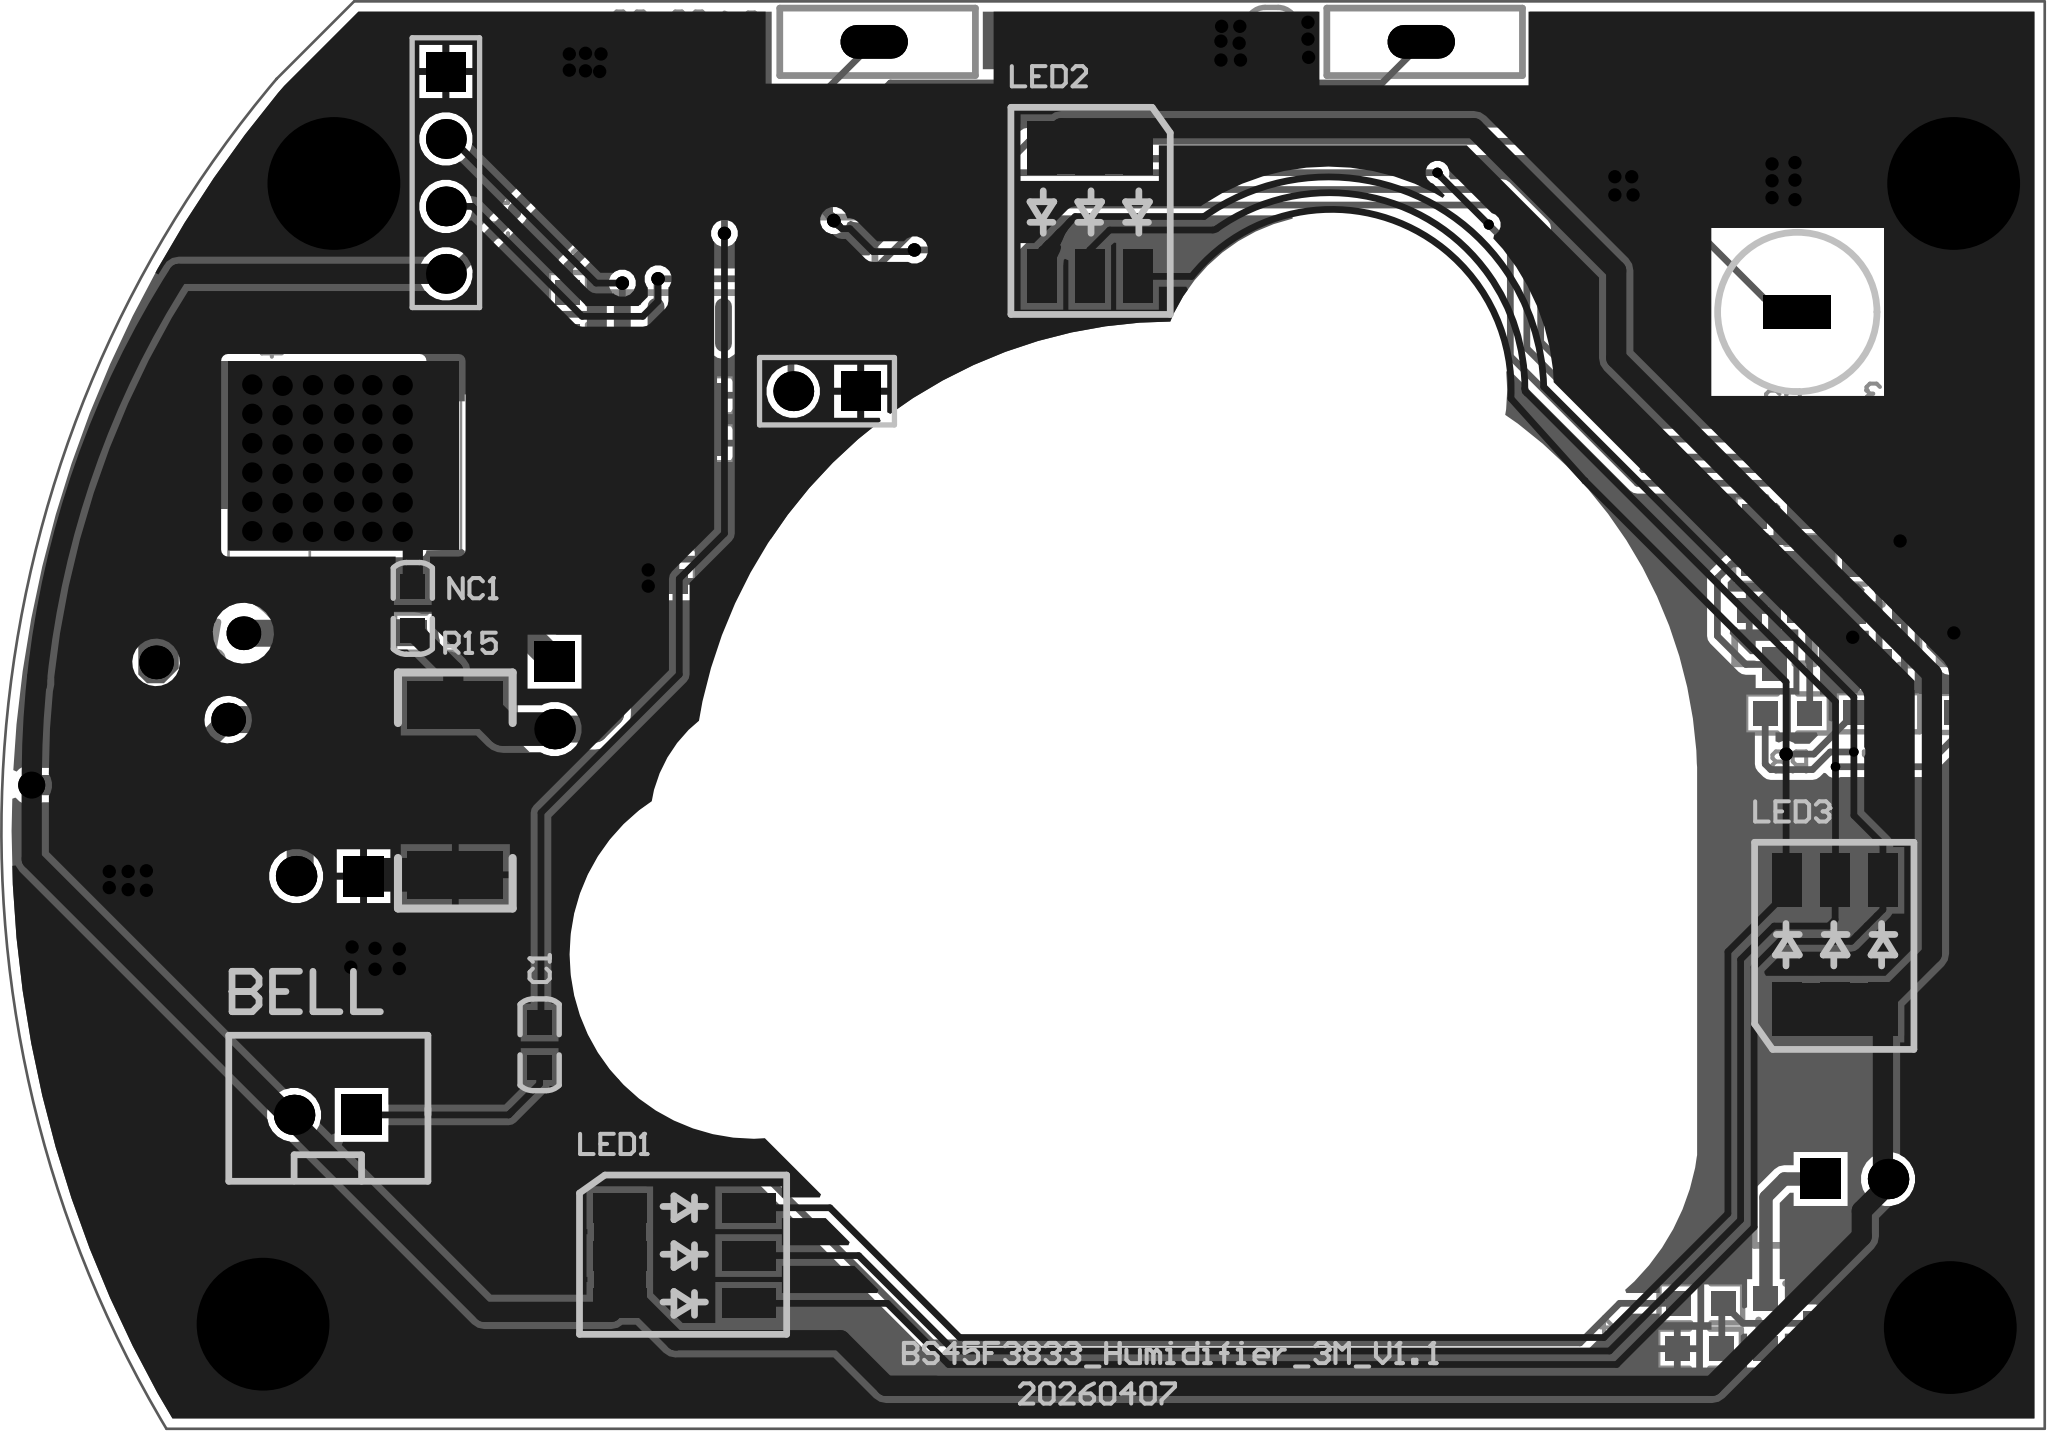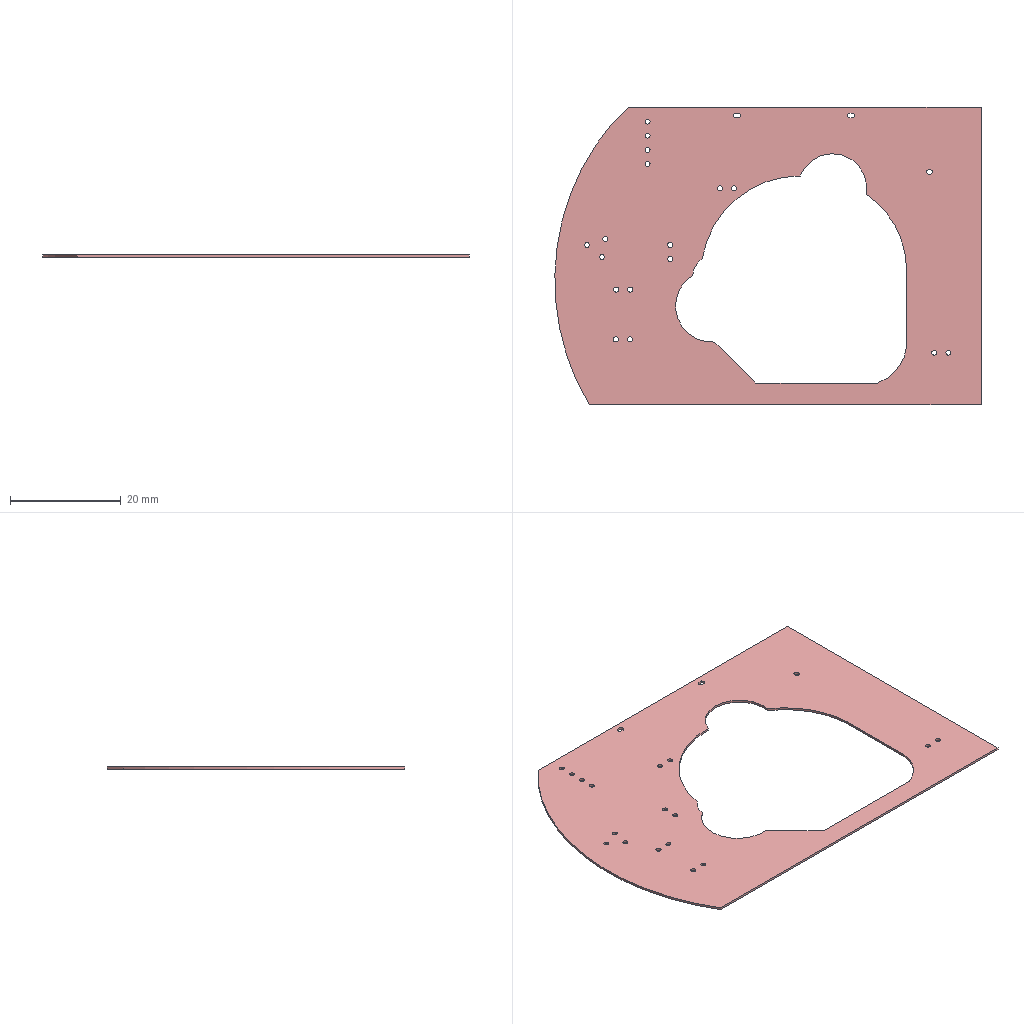Circuit board layout | Altium Designer | box 76.9 x 53.8 x 0.4 mm
Layer stack:
# Altium Designer layer stack of  (unit mm; dielectric type: 0 none, 1 core, 2 prepreg, 3 surface material)
index,name,kind,layer,copper_thickness_mm,dielectric_type,dielectric_thickness_mm,dielectric_material,dielectric_constant
0,Top Paste,other,,,,,,
1,Top Overlay,other,,,,,,
2,Top Solder,dielectric,,,3,0.0102,Solder Resist,3.5
3,Top Layer,copper,Top Layer,0.0356,,,,
4,Dielectric1,dielectric,,,0,0.32,FR-4,4.8
5,Bottom Layer,copper,Bottom Layer,0.0356,,,,
6,Bottom Solder,dielectric,,,3,0.0102,Solder Resist,3.5
7,Bottom Overlay,other,,,,,,
8,Bottom Paste,other,,,,,,
# drill layer pairs: low layer,high layer
drill_pair,Top Layer,Bottom Layer
Part placement:
Designator,Comment,Layer,Footprint,Center-X(mm),Center-Y(mm),Rotation
BELL,BELL,TopLayer,con2-wafer,873.785,988.543,180
RB2,RES,BottomLayer,0603R,877.875,1006.704,180
RB1,RES,BottomLayer,0603R,868.655,1011.123,270
C8,CAP,BottomLayer,0603C,867.054,1000.15,90
C7,CAP,BottomLayer,0603C,865.251,1000.15,90
R8,100R/1206,BottomLayer,0603R,928.747,1003.661,0
C9,22pF,BottomLayer,0603C,887.476,1015.644,180
C14,CAP,BottomLayer,0603C,874.141,1006.704,180
L1,INDUCTOR,BottomLayer,TREE,868.961,1005.056,80
雾化器,,BottomLayer,con2-wafer,882.322,1004.342,270
U1,BS45F3833_16PIN,BottomLayer,NSOP_16,889.318,1020.919,270
TX1,TX,TopLayer,HDR1X2,892.581,1015.797,180
R6,2.2K,BottomLayer,0603R,928.294,1009.294,180
R2,2.2K,BottomLayer,0603R,928.348,1011.087,180
R5,2.2K,BottomLayer,0603R,932.104,1009.269,180
R3,15R,BottomLayer,0603R,932.129,1011.301,180
R4,2.2K,BottomLayer,0603R,935.914,1009.269,180
R1,2.2K,BottomLayer,0603R,935.914,1011.276,180
R9,100R/1206,BottomLayer,0603R,935.939,1003.681,180
R7,100R/1206,BottomLayer,0603R,932.155,1003.706,0
R14,,BottomLayer,0603R,925.485,981.447,0
R15,RES,TopLayer,2512,878.586,1000.785,90
R13,RES,BottomLayer,0603R,884.123,1010.31,180
R11,RES,BottomLayer,0603R,885.8,1012.063,180
R12,RES,BottomLayer,0603R,883.285,1012.952,90
R10,RES,BottomLayer,0603R,882.828,1018.692,270
Q2,S8050,BottomLayer,SOT_23,928.261,1006.522,0
Q1,S8050,BottomLayer,SOT_23,932.198,1006.471,0
Q3,S8050,BottomLayer,SOT_23,935.957,1006.522,0
Q5,S8050,BottomLayer,SOT_23,928.954,980.694,90
Q4,NCE0110K,BottomLayer,TO252-3,877.121,1012.622,180
WATER1,WATER,TopLayer,Touch-Pad,929.118,1018.78,0
LED2,RGB,TopLayer,LED-5050,902.474,1022.545,270
LED3,RGB,TopLayer,LED-5050,930.542,994.952,90
LED1,RGB,TopLayer,LED-5050,887.205,983.246,0
ICP1,ICP,TopLayer,HDR1X4,878.23,1024.026,270
FAN1,FAN,BottomLayer,con2-wafer,931.266,986.13,0
C11,CAP,BottomLayer,0603C,886.892,1009.472,90
C10,CAP,BottomLayer,0603C,887.476,1013.841,180
C1,0.1uF,TopLayer,0603C,881.761,991.184,90
C2,0.1uF,BottomLayer,0603C,885.266,1027.151,90
C3,0.1uF,BottomLayer,0603C,887.298,1027.151,90
C12,CAP,BottomLayer,0603C,873.608,1001.141,180
1,POWER_5V,BottomLayer,con2-wafer,873.862,997.534,180
C4,CAP,BottomLayer,0603C,925.798,1023.944,180
C6,CAP,BottomLayer,0603C,889.283,1027.221,270
C5,CAP,BottomLayer,0603C,909.32,1028.522,270
NC1,CAP,TopLayer,0603C,876.986,1007.618,90
R16,2.2K,BottomLayer,0603R,925.437,979.74,0
KEY1,KEY1,BottomLayer,TP2,914.959,1028.954,0
C13,CAP,BottomLayer,0603C,873.608,1002.894,180
KEY2,KEY2,BottomLayer,TP2,894.359,1028.954,0
Pad and via stacks:
# Altium Designer via and pad stacks of  (unit mm). Each distinct definition once, with the count of objects using it.
# via: kind,start_layer,end_layer,hole_mm,diameter_mm,mode(0 simple;1 top-mid-bottom;2 full stack),diameter_per_layer,count,example_net
# pad: kind,layer,hole_mm,hole_type(0 round;1 square;2 slot),plating,top_size,top_shape(1 round;2 rect;3 octagon;9 rounded rect),mid_size,bottom_size,mode,footprint,size_per_layer,count,example
pad,Multi-Layer,0.9144,0,plated,1.524x1.524,2,1.524x1.524,1.524x1.524,0,con2-wafer,,4,BELL.1
pad,Multi-Layer,0.9144,0,plated,1.524x1.524,1,1.524x1.524,1.524x1.524,0,con2-wafer,,4,BELL.2
pad,Multi-Layer,0.889,0,plated,1.27x1.27,1,1.27x1.27,1.27x1.27,0,TREE,,3,L1.1
pad,Multi-Layer,0.9,0,plated,1.5x1.5,2,1.5x1.5,1.5x1.5,0,HDR1X2,,1,TX1.1
pad,Multi-Layer,0.9,0,plated,1.5x1.5,1,1.5x1.5,1.5x1.5,0,HDR1X2,,1,TX1.2
pad,Multi-Layer,1.016,0,plated,2.54x1.27,2,2.54x1.27,2.54x1.27,0,Touch-Pad,,1,WATER1.1
pad,Multi-Layer,0.9,0,plated,1.5x1.5,1,1.5x1.5,1.5x1.5,0,HDR1X4,,3,ICP1.4
pad,Multi-Layer,0.9,0,plated,1.5x1.5,2,1.5x1.5,1.5x1.5,0,HDR1X4,,1,ICP1.1
pad,Multi-Layer,0.889,2,plated,1.27x2.54,1,1.27x2.54,1.27x2.54,0,TP2,,2,KEY1.1
pad,Top Layer,0,0,plated,0.9144x0.9144,2,0.9144x0.9144,0.9144x0.9144,0,0603C,,4,C1.1
pad,Top Layer,0,0,plated,1.8x3.6,2,1.8x3.6,1.8x3.6,0,2512,,2,R15.1
pad,Top Layer,0,0,plated,2x1.1,2,2x1.1,2x1.1,0,LED-5050,,18,LED2.6
pad,Bottom Layer,0,0,plated,0.9144x0.9144,2,0.9144x0.9144,0.9144x0.9144,0,0603R,,34,RB1.1
pad,Bottom Layer,0,0,plated,0.9144x0.9144,2,0.9144x0.9144,0.9144x0.9144,0,0603C,,26,C8.1
pad,Bottom Layer,0,0,plated,1.27x0.9144,2,1.27x0.9144,1.27x0.9144,0,SOT_23,,4,Q3.2
pad,Bottom Layer,0,0,plated,0.9144x0.9144,2,0.9144x0.9144,0.9144x0.9144,0,SOT_23,,8,Q3.3
pad,Bottom Layer,0,0,plated,2.032x0.635,2,2.032x0.635,2.032x0.635,0,NSOP 16,,1,U1.1
pad,Bottom Layer,0,0,plated,2.032x0.635,1,2.032x0.635,2.032x0.635,0,NSOP 16,,15,U1.14
pad,Bottom Layer,0,0,plated,0.8x2.5,2,0.8x2.5,0.8x2.5,0,TO252-3,,2,Q4.3
pad,Bottom Layer,0,0,plated,5.55x6.7,2,5.55x6.7,5.55x6.7,0,TO252-3,,1,Q4.2
via,Top Layer,Bottom Layer,0.3556,0.508,0,,4,ICPCK
via,Top Layer,Bottom Layer,0.3,0.5,0,,43,GND
via,Top Layer,Bottom Layer,0.254,0.3556,0,,2,L_B
via,Top Layer,Bottom Layer,0.3556,0.5,0,,1,NetC1_2
via,Top Layer,Bottom Layer,0.254,0.381,0,,2,RGB_B
via,Top Layer,Bottom Layer,0.635,0.762,0,,36,NetNC1_2
via,Top Layer,Bottom Layer,0.7112,1.016,0,,1,+5V
via,Top Layer,Bottom Layer,4,5,0,,4,GND
Copper pours:
name,layer,net,type(0 solid;1 hatched;2 none)
GND_L01_P000,Top Layer,GND,0
GND_L02_P005,Bottom Layer,GND,0
Design rules, without the lines most boards share:
# Altium Designer design rules of  (exported by Altium Designer, unit mm)
# columns: name | kind | enabled | priority | scope1 | scope2 | descriptor | typed fields (field=value)
Clearance_10 | 0 | enabled | 1 | InNet('NetB2_1') | All | Clearance Constraint (Gap=0.635mm) (InNet('NetB2_1')),(All) | gap=0.635
Clearance_9 | 0 | enabled | 2 | InNet('NetC14_2') | All | Clearance Constraint (Gap=0.508mm) (InNet('NetC14_2')),(All) | gap=0.508
Clearance_8 | 0 | enabled | 3 | InNet('K1') | All | Clearance Constraint (Gap=0.381mm) (InNet('K1')),(All) | gap=0.381
Clearance_7 | 0 | enabled | 4 | InNet('K2') | All | Clearance Constraint (Gap=0.381mm) (InNet('K2')),(All) | gap=0.381
Clearance_6 | 0 | enabled | 5 | InNet('WATER') | All | Clearance Constraint (Gap=0.381mm) (InNet('WATER')),(All) | gap=0.381
Clearance_5 | 0 | enabled | 6 | InNet('NetB2_1') | All | Clearance Constraint (Gap=0.508mm) (InNet('NetB2_1')),(All) | gap=0.508
Clearance_4 | 0 | enabled | 7 | InNet('NetB2_2') | All | Clearance Constraint (Gap=0.508mm) (InNet('NetB2_2')),(All) | gap=0.508
Clearance_3 | 0 | enabled | 8 | InNet('NetB1_2') | All | Clearance Constraint (Gap=0.508mm) (InNet('NetB1_2')),(All) | gap=0.508
Clearance_2 | 0 | enabled | 9 | InNet('NetB1_1') | All | Clearance Constraint (Gap=0.508mm) (InNet('NetB1_1')),(All) | gap=0.508
Clearance_1 | 0 | enabled | 10 | InNet('+5V') | All | Clearance Constraint (Gap=0.254mm) (InNet('+5V')),(All) | gap=0.254
GND | 2 | enabled | 1 | InNet('GND') | All | Width Constraint (Min=0.508mm) (Max=1.524mm) (Preferred=0.508mm) (InNet('GND')) |
NetAntennae | 56 | enabled | 1 | All | All | Net Antennae (Tolerance=0mm) (All) |
SilkToSilkClearance | 55 | enabled | 1 | All | All | Silk to Silk (Clearance=0.051mm) (All),(All) |
SilkscreenOverComponentPads | 54 | enabled | 1 | IsPad | All | Silk To Solder Mask (Clearance=0.051mm) (IsPad),(All) |
MinimumSolderMaskSliver | 53 | enabled | 1 | All | All | Minimum Solder Mask Sliver (Gap=0.102mm) (All),(All) |
HoleToHoleClearance | 52 | enabled | 1 | All | All | Hole To Hole Clearance (Gap=0.152mm) (All),(All) | gap=0.1524
DiffPairsRouting | 51 | enabled | 1 | All | All | Differential Pairs Uncoupled Length using the Gap Constraints (Min=0.254mm) (Max=0.254mm) (Prefered=0.254mm)  and Width Constraints (Min=0.381mm) (Max=0.381mm) (Prefered=0.381mm) (All) |
HoleSize | 42 | enabled | 1 | All | All | Hole Size Constraint (Min=0.025mm) (Max=100mm) (All) |
Height | 50 | disabled | 1 | All | All | Height Constraint (Min=0mm) (Max=25.4mm) (Prefered=12.7mm) (Disabled)(All) | min_height=0 max_height=25.4
ComponentClearance | 24 | disabled | 1 | All | All | Component Clearance Constraint ( Horizontal Gap = 0.254mm, Vertical Gap = 0.254mm ) (Disabled)(All),(All)  | gap=0.254
SolderMaskExpansion | 13 | enabled | 1 | All | All | Solder Mask Expansion (Expansion =0.102mm) (All) | expansion=0.1016
PasteMaskExpansion | 14 | enabled | 1 | All | All | Paste Mask Expansion (Expansion =0mm) (All) | expansion=0
RoutingVias | 11 | enabled | 1 | All | All | Routing Via (MinHoleWidth=0.711mm) (MaxHoleWidth=0.711mm) (PreferredHoleWidth=0.711mm) (MinWidth=1.27mm) (MaxWidth=1.27mm) (PreferedWidth=1.27mm) (All) | via_min_hole=0.7112 via_max_hole=0.7112 via_preferred_diameter=1.27 via_preferred_hole=0.7112
RoutingCorners | 10 | enabled | 1 | All | All | Routing Corners (Style=45-Degree) (Min Setback=2.54mm) (Max Setback=2.54mm) (All) |
+5V | 2 | enabled | 2 | InNet('+5V') | All | Width Constraint (Min=0.508mm) (Max=1.524mm) (Preferred=0.762mm) (InNet('+5V')) |
PolygonConnect | 20 | enabled | 1 | All | All | Polygon Connect Rule(Relief Connect )(Conductor Width=0.254mm) (Relief Angle=90 Angle) (Entries=4) (Air Gap Width=0.254mm) (All),(All) | connect_style(0=relief,1=direct,2=none)=0 relief_conductor_width=0.254 relief_entries=4
PlaneClearance | 12 | enabled | 1 | All | All | Power Plane Clearance (Clearance =0.508mm) (All) | clearance=0.508
PlaneConnect | 6 | enabled | 1 | All | All | Power Plane Connect Rule(Relief Connect )(Expansion=0.508mm) (Conductor Width=0.254mm) (Air Gap=0.254mm) (Entries=4) (All) | relief_conductor_width=0.254 relief_entries=4 relief_expansion=0.508
Clearance | 0 | enabled | 11 | All | All | Clearance Constraint (Gap=0.254mm) (All),(All) | gap=0.254
Width_1 | 2 | enabled | 3 | All | All | Width Constraint (Min=0.254mm) (Max=1.27mm) (Preferred=0.254mm) (All) |